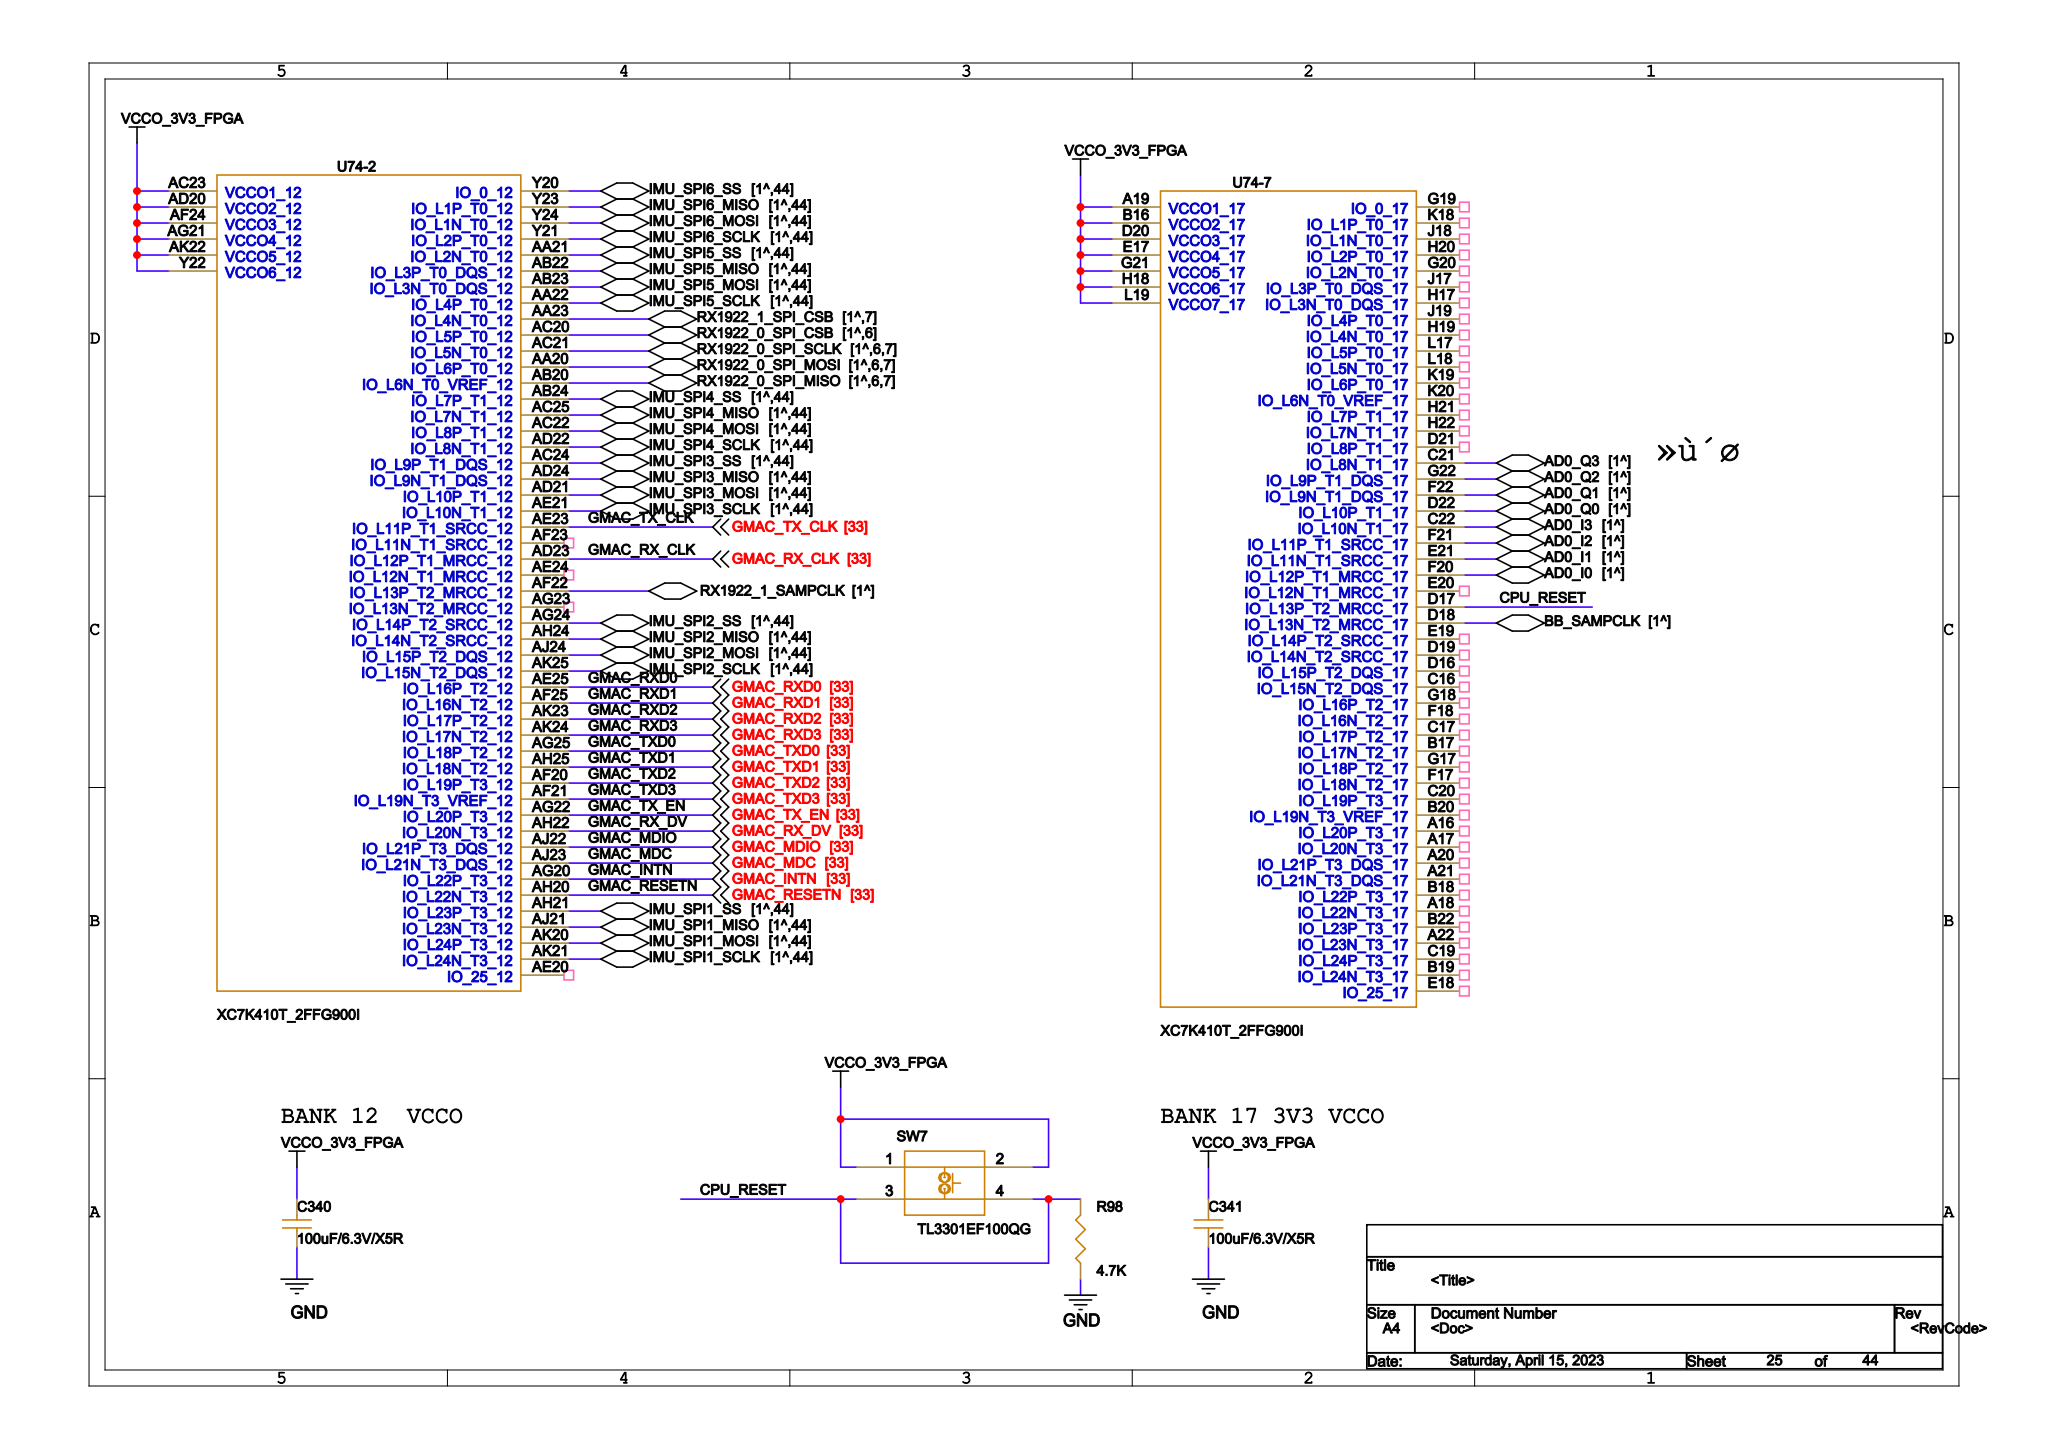Circuit board | Cadence Allegro | 1034 parts | 912 nets | one sheet of the schematic
Parts on this sheet (reference | value | footprint):
C340 | 100uF/6.3V/X5R | C0402_BGA
C341 | 100uF/6.3V/X5R | C0402_BGA
R98 | 4.7k | R0402
SW7 | TL3301EF100QG | GULLWING4
Nets of these parts (net: part-pin ...):
GND: C340-1 C341-1 R98-1
VCCO_3V3_FPGA: C340-2 C341-2 SW7-1 SW7-2
CPU_RESET: R98-2 SW7-3 SW7-4